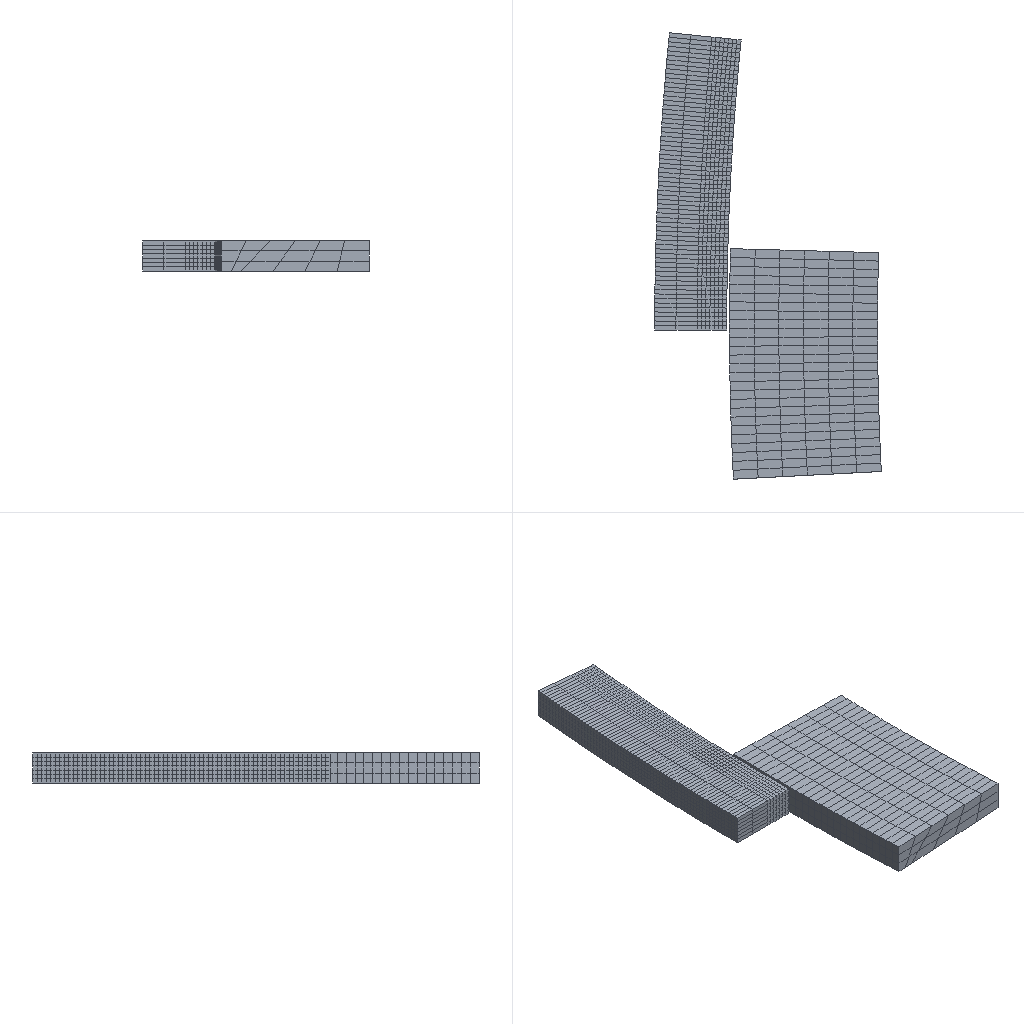Simulation study | abaqus
Set-up summary:
category,name,step,type,value,unit,region
solver,abaqus
solver,version,,,Abaqus/Explicit 2020
units,not stated in the deck,,not stated
analysis,deck,,dynamic temperature-displacement,dynamic temperature-displacement
load_step,Step-1,Step-1,dynamic temperature-displacement
load_step,requested,,,1
mesh,nodes,,,6116
mesh,elements,,,4626
element_type,C3D8T,,solid,468
element_type,C3D8RT,,solid,4158
load,load commands in deck,,count,2
bc,support commands in deck,,count,7
material,RIGID,,in results
material,STEEL,,in results
check,setup vs results,,match,"per instance, exact: element labels, types and connectivity; labels of the nodes the elements use; coordinates of those nodes at SINGLE_PRECISION in 2 of 2 instance(s)"
Abaqus input file, long lists of numbers shortened:
*Heading
** Job name: Job-1 Model name: Model-1
** Generated by: Abaqus/CAE 2020
*Preprint, echo=NO, model=NO, history=NO, contact=NO
**
** PARTS
**
*Part, name=work-1
*Node
      1,  -332.188,           0.,           0.
      2,        -337.,           0.,           0.
** (5358 more lines like these left out)
*Element, type=C3D8RT
  1,  283, 1377, 2631,  597,    1,   15,  467,  115
  2, 1377,  295,  987, 2631,   15,    2,   16,  467
** (4156 more lines like these left out)
*Nset, nset=Set-4, generate
    1,  5360,     1
*Elset, elset=Set-4, generate
    1,  4158,     1
** Section: work
*Solid Section, elset=Set-4, material=steel
,
*End Part
**
*Part, name=work-2
*Node
      1,  -310.854,   25.033,    3.4
      2,  -310.928,   24.086,    3.4
** (754 more lines like these left out)
*Element, type=C3D8T
  1,   1,   2,  29,  28, 190, 191, 218, 217
  2,   2,   3,  30,  29, 191, 192, 219, 218
** (466 more lines like these left out)
*Nset, nset=Set-1, generate
   1,  756,    1
*Elset, elset=Set-1, generate
   1,  468,    1
** Section: rigid
*Solid Section, elset=Set-1, material=rigid
,
*End Part
**
**
** ASSEMBLY
**
*Assembly, name=Assembly
**
*Instance, name=work-1-1, part=work-1
*End Instance
**
*Instance, name=work-2-1, part=work-2
          0.,           0.,           0.
          0.,           0.,           0.,           0.,           0., 1., 3.
*End Instance
**
*Node
      1,           0., 2.06352981e-14,           0.
*Nset, nset=Set-1, instance=work-1-1
    2,    3,    6,    7,   16,   17,   18,   19,   20,   21,   22,   23,   24,   25,   26,   27
   28,   29,   30,   31,   32,   33,   34,   35,   36,   37,   38,   39,   40,   41,   42,   43
** (32 more lines like these left out)
*Elset, elset=Set-1, instance=work-1-1, generate
   2,  924,    2
*Nset, nset=Set-4
 1,
*Nset, nset=Set-5
 1,
*Nset, nset=Set-6, instance=work-1-1, generate
    1,  5360,     1
*Nset, nset=Set-6, instance=work-2-1, generate
   1,  756,    1
*Elset, elset=Set-6, instance=work-1-1, generate
    1,  4158,     1
*Elset, elset=Set-6, instance=work-2-1, generate
   1,  468,    1
*Nset, nset=b_Set-2, instance=work-2-1, generate
   1,  756,    1
*Elset, elset=b_Set-2, instance=work-2-1, generate
   1,  468,    1
*Nset, nset=s_Set-7, instance=work-1-1
    1,    4,    5,    8,    9,   10,   11,   12,   13,   14,   82,   83,   84,   85,   86,   87
   88,   89,   90,   91,   92,   93,   94,   95,   96,   97,   98,   99,  100,  101,  102,  103
** (266 more lines like these left out)
*Elset, elset=s_Set-7, instance=work-1-1, generate
  925,  4158,     1
*Nset, nset=_PickedSet10, internal
 1,
*Elset, elset=_m_Surf-1_S4, internal, instance=work-2-1, generate
  26,  468,   26
*Elset, elset=_m_Surf-1_S1, internal, instance=work-2-1, generate
   1,  156,    1
*Elset, elset=_m_Surf-1_S6, internal, instance=work-2-1, generate
   1,  443,   26
*Elset, elset=_m_Surf-1_S5, internal, instance=work-2-1
 131, 132, 133, 134, 135, 136, 137, 138, 139, 140, 141, 142, 143, 144, 145, 146
 147, 148, 149, 150, 151, 152, 153, 154, 155, 156, 287, 288, 289, 290, 291, 292
** (3 more lines like these left out)
*Elset, elset=_m_Surf-1_S2, internal, instance=work-2-1, generate
 313,  468,    1
*Surface, type=ELEMENT, name=m_Surf-1
_m_Surf-1_S4, S4
_m_Surf-1_S1, S1
_m_Surf-1_S6, S6
_m_Surf-1_S2, S2
_m_Surf-1_S5, S5
*Elset, elset=_s_Surf-1_S6, internal, instance=work-1-1, generate
  925,  4093,    66
*Elset, elset=_s_Surf-1_S3, internal, instance=work-1-1
    1,    2,  133,  134,  265,  266,  397,  398,  529,  530,  661,  662,  793,  794,  925,  926
  927,  928,  929,  930,  931,  932,  933,  934,  935,  936,  937,  938,  939,  940,  941,  942
** (28 more lines like these left out)
*Elset, elset=_s_Surf-1_S5, internal, instance=work-1-1
  131,  132,  263,  264,  395,  396,  527,  528,  659,  660,  791,  792,  923,  924, 1321, 1322
 1323, 1324, 1325, 1326, 1327, 1328, 1329, 1330, 1331, 1332, 1333, 1334, 1335, 1336, 1337, 1338
** (28 more lines like these left out)
*Elset, elset=_s_Surf-1_S4, internal, instance=work-1-1, generate
  990,  4158,    66
*Elset, elset=_s_Surf-1_S1, internal, instance=work-1-1
  793,  794,  795,  796,  797,  798,  799,  800,  801,  802,  803,  804,  805,  806,  807,  808
  809,  810,  811,  812,  813,  814,  815,  816,  817,  818,  819,  820,  821,  822,  823,  824
** (36 more lines like these left out)
*Elset, elset=_s_Surf-1_S2, internal, instance=work-1-1, generate
   1,  132,    1
*Surface, type=ELEMENT, name=s_Surf-1
_s_Surf-1_S6, S6
_s_Surf-1_S3, S3
_s_Surf-1_S4, S4
_s_Surf-1_S2, S2
_s_Surf-1_S5, S5
_s_Surf-1_S1, S1
*Surface, type=NODE, name=s_Set-7_CNS_, internal
s_Set-7, 1.
** Constraint: Constraint-1
*Rigid Body, ref node=_PickedSet10, elset=b_Set-2
*End Assembly
*Amplitude, name=Amp-1
             0.,              0.,           0.005,              1.,            0.01,             -1.,           0.015,              1.
           0.02,             -1.,           0.025,              1.,            0.03,             -1.,           0.035,              1.
           0.04,             -1.,           0.045,              1.,            0.05,             -1.,           0.055,              1.
           0.06,             -1.,           0.065,              1.,            0.07,             -1.,           0.075,              1.
           0.08,             -1.,           0.085,              1.,            0.09,             -1.,           0.095,              1.
            0.1,             -1.
**
** MATERIALS
**
*Material, name=rigid
*Conductivity
44.,
*Density
 7.82e-09,
*Elastic
206000., 0.29
*Expansion
 1.3e-05,
*Specific Heat
 4.6e+08,
*Material, name=steel
*Conductivity
44.,   0.
60.,1000.
*Damage Initiation, criterion=SHEAR
2.,0.,0.
*Damage Evolution, type=DISPLACEMENT
 0.001,
*Density
 7.82e-09,
*Elastic
206000., 0.29
*Expansion
 1.3e-10,
*Inelastic Heat Fraction
         0.9,
*Plastic
400.,   0.,  20.
320.,   0., 100.
250.,   0., 300.
 20.,   0.,1500.
*Specific Heat
 4.6e+08,
**
** INTERACTION PROPERTIES
**
*Surface Interaction, name=IntProp-1
*Friction
 0.2,
*Surface Behavior, pressure-overclosure=HARD
*Gap Conductance
 0.5,  0.
  0., 0.1
**
** PREDEFINED FIELDS
**
** Name: Predefined Field-1   Type: Temperature
*Initial Conditions, type=TEMPERATURE
Set-6, 20.
** ----------------------------------------------------------------
**
** STEP: Step-1
**
*Step, name=Step-1, nlgeom=YES
*Dynamic Temperature-displacement, Explicit
, 0.1
*Bulk Viscosity
0.06, 1.2
** Mass Scaling: Semi-Automatic
**               Whole Model
*Fixed Mass Scaling, factor=500.
**
** BOUNDARY CONDITIONS
**
** Name: BC-1 Type: 对称/反对称/完全固定
*Boundary
Set-1, ENCASTRE
** Name: [REDACTED] : Velocity/Angular velocity
*Boundary, type=VELOCITY
Set-5, 1, 1, -20.
Set-5, 2, 2
Set-5, 3, 3
Set-5, 4, 4
Set-5, 5, 5
** Name: [REDACTED] : Velocity/Angular velocity
*Boundary, amplitude=Amp-1, type=VELOCITY
Set-4, 6, 6, -23.
**
** INTERACTIONS
**
** Interaction: Int-1
*Contact Pair, interaction=IntProp-1, mechanical constraint=KINEMATIC, cpset=Int-1
m_Surf-1, s_Set-7_CNS_
**
** OUTPUT REQUESTS
**
*Restart, write, number interval=1, time marks=NO
**
** FIELD OUTPUT: F-Output-1
**
*Output, field, number interval=240
*Node Output
A, NT, RF, RFL, RM, RT, U, V
*Element Output, directions=YES
E, HFL, LE, MISES, PE, PEEQ, PEEQVAVG, PEVAVG, S, STATUS, SVAVG, TEMP
*Contact Output
CDISP, CSTRESS
**
** HISTORY OUTPUT: H-Output-1
**
*Output, history, time interval=5e-05
*Node Output, nset=Set-5
RF1, RF2, RF3, RM1, RM2, RM3
*End Step
Results summary:
result,step,Step-1,completed,increments=194743 time=0.1/0.1
result,analysis,,,"dynamic temperature-displacement, explict"
result,last_loadstep,,,1
result,primary field,,,"U, NT11"
result,reaction total,,FX,5017.763,model units
result,reaction total,,FY,-17211.938,model units
result,reaction total,,FZ,-52.257,model units